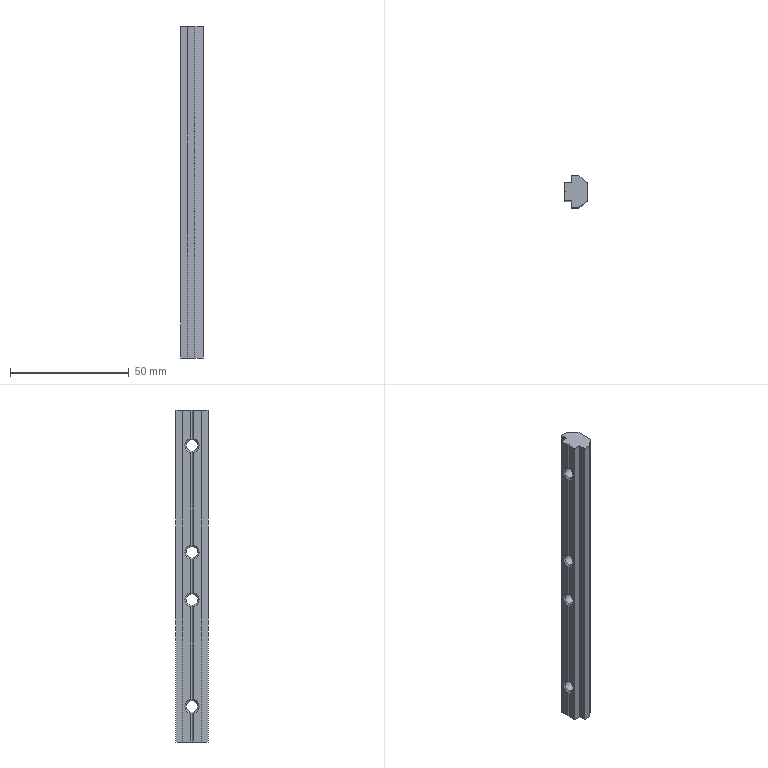Part | SolidWorks | features BaseBody 1 | 1 solid | 47 faces | box 9.5 x 13.5 x 140 mm | volume 13278 mm3 | plane 23 | cone 16 | cylinder 8 | commonest cylinder face diameters 4.917 x8
STEP:
#1=CARTESIAN_POINT('',(-0.5415,0.,-12.542));
#2=VERTEX_POINT('',#1);
#3=CARTESIAN_POINT('',(-0.5415,0.,-17.458));
#4=VERTEX_POINT('',#3);
#5=CARTESIAN_POINT('',(-0.5415,0.,-15.));
#6=DIRECTION('',(1.,0.,0.));
#7=DIRECTION('',(0.,0.,-1.));
#8=AXIS2_PLACEMENT_3D('',#5,#6,#7);
#9=CIRCLE('',#8,2.458);
#10=EDGE_CURVE('',#2,#4,#9,.T.);
#11=ORIENTED_EDGE('',*,*,#10,.F.);
#12=CARTESIAN_POINT('',(0.,0.,-12.));
#13=VERTEX_POINT('',#12);
#14=CARTESIAN_POINT('',(0.,0.,-12.));
#15=DIRECTION('',(0.7071,0.,0.7071));
#16=VECTOR('',#15,1000.);
#17=LINE('',#14,#16);
#18=EDGE_CURVE('',#2,#13,#17,.T.);
#19=ORIENTED_EDGE('',*,*,#18,.T.);
#20=CARTESIAN_POINT('',(0.,0.,-18.));
#21=VERTEX_POINT('',#20);
#22=CARTESIAN_POINT('',(0.,0.,-15.));
#23=DIRECTION('',(-1.,0.,0.));
#24=DIRECTION('',(0.,0.,-1.));
#25=AXIS2_PLACEMENT_3D('',#22,#23,#24);
#26=CIRCLE('',#25,3.);
#27=EDGE_CURVE('',#21,#13,#26,.T.);
#28=ORIENTED_EDGE('',*,*,#27,.F.);
#29=CARTESIAN_POINT('',(0.,0.,-18.));
#30=DIRECTION('',(0.7071,0.,-0.7071));
#31=VECTOR('',#30,1000.);
#32=LINE('',#29,#31);
#33=EDGE_CURVE('',#4,#21,#32,.T.);
#34=ORIENTED_EDGE('',*,*,#33,.F.);
#35=EDGE_LOOP('',(#11,#19,#28,#34));
#36=FACE_OUTER_BOUND('',#35,.T.);
#37=CARTESIAN_POINT('',(0.,0.,-15.));
#38=DIRECTION('',(1.,0.,0.));
#39=DIRECTION('',(0.,0.,-1.));
#40=AXIS2_PLACEMENT_3D('',#37,#38,#39);
#41=CONICAL_SURFACE('',#40,3.,0.7854);
#42=ADVANCED_FACE('',(#36),#41,.F.);
#43=CARTESIAN_POINT('',(-0.5415,0.,-57.541));
#44=VERTEX_POINT('',#43);
#45=CARTESIAN_POINT('',(-0.5415,0.,-62.459));
#46=VERTEX_POINT('',#45);
#47=CARTESIAN_POINT('',(-0.5415,0.,-60.));
#48=DIRECTION('',(1.,0.,0.));
#49=DIRECTION('',(0.,0.,-1.));
#50=AXIS2_PLACEMENT_3D('',#47,#48,#49);
#51=CIRCLE('',#50,2.459);
#52=EDGE_CURVE('',#44,#46,#51,.T.);
#53=ORIENTED_EDGE('',*,*,#52,.F.);
#54=CARTESIAN_POINT('',(0.,0.,-57.));
#55=VERTEX_POINT('',#54);
#56=CARTESIAN_POINT('',(0.,0.,-57.));
#57=DIRECTION('',(0.7071,0.,0.7071));
#58=VECTOR('',#57,1000.);
#59=LINE('',#56,#58);
#60=EDGE_CURVE('',#44,#55,#59,.T.);
#61=ORIENTED_EDGE('',*,*,#60,.T.);
#62=CARTESIAN_POINT('',(0.,0.,-63.));
#63=VERTEX_POINT('',#62);
#64=CARTESIAN_POINT('',(0.,0.,-60.));
#65=DIRECTION('',(-1.,0.,0.));
#66=DIRECTION('',(0.,0.,-1.));
#67=AXIS2_PLACEMENT_3D('',#64,#65,#66);
#68=CIRCLE('',#67,3.);
#69=EDGE_CURVE('',#63,#55,#68,.T.);
#70=ORIENTED_EDGE('',*,*,#69,.F.);
#71=CARTESIAN_POINT('',(0.,0.,-63.));
#72=DIRECTION('',(0.7071,0.,-0.7071));
#73=VECTOR('',#72,1000.);
#74=LINE('',#71,#73);
#75=EDGE_CURVE('',#46,#63,#74,.T.);
#76=ORIENTED_EDGE('',*,*,#75,.F.);
#77=EDGE_LOOP('',(#53,#61,#70,#76));
#78=FACE_OUTER_BOUND('',#77,.T.);
#79=CARTESIAN_POINT('',(0.,0.,-60.));
#80=DIRECTION('',(1.,0.,0.));
#81=DIRECTION('',(0.,0.,-1.));
#82=AXIS2_PLACEMENT_3D('',#79,#80,#81);
#83=CONICAL_SURFACE('',#82,3.,0.7854);
#84=ADVANCED_FACE('',(#78),#83,.F.);
#85=CARTESIAN_POINT('',(-0.5415,0.,-77.542));
#86=VERTEX_POINT('',#85);
#87=CARTESIAN_POINT('',(-0.5415,0.,-82.458));
#88=VERTEX_POINT('',#87);
#89=CARTESIAN_POINT('',(-0.5415,0.,-80.));
#90=DIRECTION('',(1.,0.,0.));
#91=DIRECTION('',(0.,0.,-1.));
#92=AXIS2_PLACEMENT_3D('',#89,#90,#91);
#93=CIRCLE('',#92,2.458);
#94=EDGE_CURVE('',#86,#88,#93,.T.);
#95=ORIENTED_EDGE('',*,*,#94,.F.);
#96=CARTESIAN_POINT('',(0.,0.,-77.));
#97=VERTEX_POINT('',#96);
#98=CARTESIAN_POINT('',(0.,0.,-77.));
#99=DIRECTION('',(0.7071,0.,0.7071));
#100=VECTOR('',#99,1000.);
#101=LINE('',#98,#100);
#102=EDGE_CURVE('',#86,#97,#101,.T.);
#103=ORIENTED_EDGE('',*,*,#102,.T.);
#104=CARTESIAN_POINT('',(0.,0.,-83.));
#105=VERTEX_POINT('',#104);
#106=CARTESIAN_POINT('',(0.,0.,-80.));
#107=DIRECTION('',(-1.,0.,0.));
#108=DIRECTION('',(0.,0.,-1.));
#109=AXIS2_PLACEMENT_3D('',#106,#107,#108);
#110=CIRCLE('',#109,3.);
#111=EDGE_CURVE('',#105,#97,#110,.T.);
#112=ORIENTED_EDGE('',*,*,#111,.F.);
#113=CARTESIAN_POINT('',(0.,0.,-83.));
#114=DIRECTION('',(0.7071,0.,-0.7071));
#115=VECTOR('',#114,1000.);
#116=LINE('',#113,#115);
#117=EDGE_CURVE('',#88,#105,#116,.T.);
#118=ORIENTED_EDGE('',*,*,#117,.F.);
#119=EDGE_LOOP('',(#95,#103,#112,#118));
#120=FACE_OUTER_BOUND('',#119,.T.);
#121=CARTESIAN_POINT('',(0.,0.,-80.));
#122=DIRECTION('',(1.,0.,0.));
#123=DIRECTION('',(0.,0.,-1.));
#124=AXIS2_PLACEMENT_3D('',#121,#122,#123);
#125=CONICAL_SURFACE('',#124,3.,0.7854);
#126=ADVANCED_FACE('',(#120),#125,.F.);
#127=CARTESIAN_POINT('',(-0.5415,0.,-122.541));
#128=VERTEX_POINT('',#127);
#129=CARTESIAN_POINT('',(-0.5415,0.,-127.459));
#130=VERTEX_POINT('',#129);
#131=CARTESIAN_POINT('',(-0.5415,0.,-125.));
#132=DIRECTION('',(1.,0.,0.));
#133=DIRECTION('',(0.,0.,-1.));
#134=AXIS2_PLACEMENT_3D('',#131,#132,#133);
#135=CIRCLE('',#134,2.459);
#136=EDGE_CURVE('',#128,#130,#135,.T.);
#137=ORIENTED_EDGE('',*,*,#136,.F.);
#138=CARTESIAN_POINT('',(0.,0.,-122.));
#139=VERTEX_POINT('',#138);
#140=CARTESIAN_POINT('',(0.,0.,-122.));
#141=DIRECTION('',(0.7071,0.,0.7071));
#142=VECTOR('',#141,1000.);
#143=LINE('',#140,#142);
#144=EDGE_CURVE('',#128,#139,#143,.T.);
#145=ORIENTED_EDGE('',*,*,#144,.T.);
#146=CARTESIAN_POINT('',(0.,0.,-128.));
#147=VERTEX_POINT('',#146);
#148=CARTESIAN_POINT('',(0.,0.,-125.));
#149=DIRECTION('',(-1.,0.,0.));
#150=DIRECTION('',(0.,0.,-1.));
#151=AXIS2_PLACEMENT_3D('',#148,#149,#150);
#152=CIRCLE('',#151,3.);
#153=EDGE_CURVE('',#147,#139,#152,.T.);
#154=ORIENTED_EDGE('',*,*,#153,.F.);
#155=CARTESIAN_POINT('',(0.,0.,-128.));
#156=DIRECTION('',(0.7071,0.,-0.7071));
#157=VECTOR('',#156,1000.);
#158=LINE('',#155,#157);
#159=EDGE_CURVE('',#130,#147,#158,.T.);
#160=ORIENTED_EDGE('',*,*,#159,.F.);
#161=EDGE_LOOP('',(#137,#145,#154,#160));
#162=FACE_OUTER_BOUND('',#161,.T.);
#163=CARTESIAN_POINT('',(0.,0.,-125.));
#164=DIRECTION('',(1.,0.,0.));
#165=DIRECTION('',(0.,0.,-1.));
#166=AXIS2_PLACEMENT_3D('',#163,#164,#165);
#167=CONICAL_SURFACE('',#166,3.,0.7854);
#168=ADVANCED_FACE('',(#162),#167,.F.);
#169=ORIENTED_EDGE('',*,*,#10,.T.);
#170=CARTESIAN_POINT('',(-8.959,0.,-17.458));
#171=VERTEX_POINT('',#170);
#172=CARTESIAN_POINT('',(0.,0.,-17.458));
#173=DIRECTION('',(-1.,0.,0.));
#174=VECTOR('',#173,1000.);
#175=LINE('',#172,#174);
#176=EDGE_CURVE('',#4,#171,#175,.T.);
#177=ORIENTED_EDGE('',*,*,#176,.T.);
#178=CARTESIAN_POINT('',(-8.959,0.,-12.542));
#179=VERTEX_POINT('',#178);
#180=CARTESIAN_POINT('',(-8.959,0.,-15.));
#181=DIRECTION('',(1.,0.,0.));
#182=DIRECTION('',(0.,0.,1.));
#183=AXIS2_PLACEMENT_3D('',#180,#181,#182);
#184=CIRCLE('',#183,2.458);
#185=EDGE_CURVE('',#179,#171,#184,.T.);
#186=ORIENTED_EDGE('',*,*,#185,.F.);
#187=CARTESIAN_POINT('',(0.,0.,-12.542));
#188=DIRECTION('',(-1.,0.,0.));
#189=VECTOR('',#188,1000.);
#190=LINE('',#187,#189);
#191=EDGE_CURVE('',#2,#179,#190,.T.);
#192=ORIENTED_EDGE('',*,*,#191,.F.);
#193=EDGE_LOOP('',(#169,#177,#186,#192));
#194=FACE_OUTER_BOUND('',#193,.T.);
#195=CARTESIAN_POINT('',(0.,0.,-15.));
#196=DIRECTION('',(-1.,0.,0.));
#197=DIRECTION('',(0.,0.,1.));
#198=AXIS2_PLACEMENT_3D('',#195,#196,#197);
#199=CYLINDRICAL_SURFACE('',#198,2.458);
#200=ADVANCED_FACE('',(#194),#199,.F.);
#201=ORIENTED_EDGE('',*,*,#52,.T.);
#202=CARTESIAN_POINT('',(-8.959,0.,-62.459));
#203=VERTEX_POINT('',#202);
#204=CARTESIAN_POINT('',(0.,0.,-62.459));
#205=DIRECTION('',(-1.,0.,0.));
#206=VECTOR('',#205,1000.);
#207=LINE('',#204,#206);
#208=EDGE_CURVE('',#46,#203,#207,.T.);
#209=ORIENTED_EDGE('',*,*,#208,.T.);
#210=CARTESIAN_POINT('',(-8.959,0.,-57.541));
#211=VERTEX_POINT('',#210);
#212=CARTESIAN_POINT('',(-8.959,0.,-60.));
#213=DIRECTION('',(1.,0.,0.));
#214=DIRECTION('',(0.,0.,1.));
#215=AXIS2_PLACEMENT_3D('',#212,#213,#214);
#216=CIRCLE('',#215,2.459);
#217=EDGE_CURVE('',#211,#203,#216,.T.);
#218=ORIENTED_EDGE('',*,*,#217,.F.);
#219=CARTESIAN_POINT('',(0.,0.,-57.541));
#220=DIRECTION('',(-1.,0.,0.));
#221=VECTOR('',#220,1000.);
#222=LINE('',#219,#221);
#223=EDGE_CURVE('',#44,#211,#222,.T.);
#224=ORIENTED_EDGE('',*,*,#223,.F.);
#225=EDGE_LOOP('',(#201,#209,#218,#224));
#226=FACE_OUTER_BOUND('',#225,.T.);
#227=CARTESIAN_POINT('',(0.,0.,-60.));
#228=DIRECTION('',(-1.,0.,0.));
#229=DIRECTION('',(0.,0.,1.));
#230=AXIS2_PLACEMENT_3D('',#227,#228,#229);
#231=CYLINDRICAL_SURFACE('',#230,2.459);
#232=ADVANCED_FACE('',(#226),#231,.F.);
#233=ORIENTED_EDGE('',*,*,#94,.T.);
#234=CARTESIAN_POINT('',(-8.959,0.,-82.459));
#235=VERTEX_POINT('',#234);
#236=CARTESIAN_POINT('',(0.,0.,-82.459));
#237=DIRECTION('',(-1.,0.,0.));
#238=VECTOR('',#237,1000.);
#239=LINE('',#236,#238);
#240=EDGE_CURVE('',#88,#235,#239,.T.);
#241=ORIENTED_EDGE('',*,*,#240,.T.);
#242=CARTESIAN_POINT('',(-8.959,0.,-77.541));
#243=VERTEX_POINT('',#242);
#244=CARTESIAN_POINT('',(-8.959,0.,-80.));
#245=DIRECTION('',(1.,0.,0.));
#246=DIRECTION('',(0.,0.,1.));
#247=AXIS2_PLACEMENT_3D('',#244,#245,#246);
#248=CIRCLE('',#247,2.459);
#249=EDGE_CURVE('',#243,#235,#248,.T.);
#250=ORIENTED_EDGE('',*,*,#249,.F.);
#251=CARTESIAN_POINT('',(0.,0.,-77.541));
#252=DIRECTION('',(-1.,0.,0.));
#253=VECTOR('',#252,1000.);
#254=LINE('',#251,#253);
#255=EDGE_CURVE('',#86,#243,#254,.T.);
#256=ORIENTED_EDGE('',*,*,#255,.F.);
#257=EDGE_LOOP('',(#233,#241,#250,#256));
#258=FACE_OUTER_BOUND('',#257,.T.);
#259=CARTESIAN_POINT('',(0.,0.,-80.));
#260=DIRECTION('',(-1.,0.,0.));
#261=DIRECTION('',(0.,0.,1.));
#262=AXIS2_PLACEMENT_3D('',#259,#260,#261);
#263=CYLINDRICAL_SURFACE('',#262,2.459);
#264=ADVANCED_FACE('',(#258),#263,.F.);
#265=ORIENTED_EDGE('',*,*,#136,.T.);
#266=CARTESIAN_POINT('',(-8.959,0.,-127.459));
#267=VERTEX_POINT('',#266);
#268=CARTESIAN_POINT('',(0.,0.,-127.459));
#269=DIRECTION('',(-1.,0.,0.));
#270=VECTOR('',#269,1000.);
#271=LINE('',#268,#270);
#272=EDGE_CURVE('',#130,#267,#271,.T.);
#273=ORIENTED_EDGE('',*,*,#272,.T.);
#274=CARTESIAN_POINT('',(-8.959,0.,-122.541));
#275=VERTEX_POINT('',#274);
#276=CARTESIAN_POINT('',(-8.959,0.,-125.));
#277=DIRECTION('',(1.,0.,0.));
#278=DIRECTION('',(0.,0.,1.));
#279=AXIS2_PLACEMENT_3D('',#276,#277,#278);
#280=CIRCLE('',#279,2.459);
#281=EDGE_CURVE('',#275,#267,#280,.T.);
#282=ORIENTED_EDGE('',*,*,#281,.F.);
#283=CARTESIAN_POINT('',(0.,0.,-122.541));
#284=DIRECTION('',(-1.,0.,0.));
#285=VECTOR('',#284,1000.);
#286=LINE('',#283,#285);
#287=EDGE_CURVE('',#128,#275,#286,.T.);
#288=ORIENTED_EDGE('',*,*,#287,.F.);
#289=EDGE_LOOP('',(#265,#273,#282,#288));
#290=FACE_OUTER_BOUND('',#289,.T.);
#291=CARTESIAN_POINT('',(0.,0.,-125.));
#292=DIRECTION('',(-1.,0.,0.));
#293=DIRECTION('',(0.,0.,1.));
#294=AXIS2_PLACEMENT_3D('',#291,#292,#293);
#295=CYLINDRICAL_SURFACE('',#294,2.459);
#296=ADVANCED_FACE('',(#290),#295,.F.);
#297=ORIENTED_EDGE('',*,*,#249,.T.);
#298=CARTESIAN_POINT('',(-9.,0.,-82.5));
#299=VERTEX_POINT('',#298);
#300=CARTESIAN_POINT('',(-9.5,0.,-83.));
#301=DIRECTION('',(-0.7071,0.,-0.7071));
#302=VECTOR('',#301,1000.);
#303=LINE('',#300,#302);
#304=EDGE_CURVE('',#235,#299,#303,.T.);
#305=ORIENTED_EDGE('',*,*,#304,.T.);
#306=CARTESIAN_POINT('',(-9.5,-0.5,-82.958));
#307=VERTEX_POINT('',#306);
#308=CARTESIAN_POINT('',(-9.5,-0.5,-82.958));
#309=CARTESIAN_POINT('',(-9.319,-0.3193,-82.805));
#310=CARTESIAN_POINT('',(-9.153,-0.1527,-82.653));
#311=CARTESIAN_POINT('',(-9.,0.,-82.5));
#312=B_SPLINE_CURVE_WITH_KNOTS('',3,(#308,#309,#310,#311),.UNSPECIFIED.,.F.,.F.,(4,4),(0.,1.),.UNSPECIFIED.);
#313=EDGE_CURVE('',#307,#299,#312,.T.);
#314=ORIENTED_EDGE('',*,*,#313,.F.);
#315=CARTESIAN_POINT('',(-9.5,-0.5,-77.042));
#316=VERTEX_POINT('',#315);
#317=CARTESIAN_POINT('',(-9.5,0.,-80.));
#318=DIRECTION('',(1.,0.,0.));
#319=DIRECTION('',(0.,0.,1.));
#320=AXIS2_PLACEMENT_3D('',#317,#318,#319);
#321=CIRCLE('',#320,3.);
#322=EDGE_CURVE('',#316,#307,#321,.T.);
#323=ORIENTED_EDGE('',*,*,#322,.F.);
#324=CARTESIAN_POINT('',(-9.,0.,-77.5));
#325=VERTEX_POINT('',#324);
#326=CARTESIAN_POINT('',(-9.,0.,-77.5));
#327=CARTESIAN_POINT('',(-9.153,-0.1527,-77.347));
#328=CARTESIAN_POINT('',(-9.319,-0.3193,-77.195));
#329=CARTESIAN_POINT('',(-9.5,-0.5,-77.042));
#330=B_SPLINE_CURVE_WITH_KNOTS('',3,(#326,#327,#328,#329),.UNSPECIFIED.,.F.,.F.,(4,4),(0.,1.),.UNSPECIFIED.);
#331=EDGE_CURVE('',#325,#316,#330,.T.);
#332=ORIENTED_EDGE('',*,*,#331,.F.);
#333=CARTESIAN_POINT('',(-9.5,0.,-77.));
#334=DIRECTION('',(-0.7071,0.,0.7071));
#335=VECTOR('',#334,1000.);
#336=LINE('',#333,#335);
#337=EDGE_CURVE('',#243,#325,#336,.T.);
#338=ORIENTED_EDGE('',*,*,#337,.F.);
#339=EDGE_LOOP('',(#297,#305,#314,#323,#332,#338));
#340=FACE_OUTER_BOUND('',#339,.T.);
#341=CARTESIAN_POINT('',(-9.5,0.,-80.));
#342=DIRECTION('',(-1.,0.,0.));
#343=DIRECTION('',(0.,0.,1.));
#344=AXIS2_PLACEMENT_3D('',#341,#342,#343);
#345=CONICAL_SURFACE('',#344,3.,0.7854);
#346=ADVANCED_FACE('',(#340),#345,.F.);
#347=ORIENTED_EDGE('',*,*,#217,.T.);
#348=CARTESIAN_POINT('',(-9.,0.,-62.5));
#349=VERTEX_POINT('',#348);
#350=CARTESIAN_POINT('',(-9.5,0.,-63.));
#351=DIRECTION('',(-0.7071,0.,-0.7071));
#352=VECTOR('',#351,1000.);
#353=LINE('',#350,#352);
#354=EDGE_CURVE('',#203,#349,#353,.T.);
#355=ORIENTED_EDGE('',*,*,#354,.T.);
#356=CARTESIAN_POINT('',(-9.5,-0.5,-62.958));
#357=VERTEX_POINT('',#356);
#358=CARTESIAN_POINT('',(-9.5,-0.5,-62.958));
#359=CARTESIAN_POINT('',(-9.319,-0.3193,-62.805));
#360=CARTESIAN_POINT('',(-9.153,-0.1527,-62.653));
#361=CARTESIAN_POINT('',(-9.,0.,-62.5));
#362=B_SPLINE_CURVE_WITH_KNOTS('',3,(#358,#359,#360,#361),.UNSPECIFIED.,.F.,.F.,(4,4),(0.,1.),.UNSPECIFIED.);
#363=EDGE_CURVE('',#357,#349,#362,.T.);
#364=ORIENTED_EDGE('',*,*,#363,.F.);
#365=CARTESIAN_POINT('',(-9.5,-0.5,-57.042));
#366=VERTEX_POINT('',#365);
#367=CARTESIAN_POINT('',(-9.5,0.,-60.));
#368=DIRECTION('',(1.,0.,0.));
#369=DIRECTION('',(0.,0.,1.));
#370=AXIS2_PLACEMENT_3D('',#367,#368,#369);
#371=CIRCLE('',#370,3.);
#372=EDGE_CURVE('',#366,#357,#371,.T.);
#373=ORIENTED_EDGE('',*,*,#372,.F.);
#374=CARTESIAN_POINT('',(-9.,0.,-57.5));
#375=VERTEX_POINT('',#374);
#376=CARTESIAN_POINT('',(-9.,0.,-57.5));
#377=CARTESIAN_POINT('',(-9.153,-0.1527,-57.347));
#378=CARTESIAN_POINT('',(-9.319,-0.3193,-57.195));
#379=CARTESIAN_POINT('',(-9.5,-0.5,-57.042));
#380=B_SPLINE_CURVE_WITH_KNOTS('',3,(#376,#377,#378,#379),.UNSPECIFIED.,.F.,.F.,(4,4),(0.,1.),.UNSPECIFIED.);
#381=EDGE_CURVE('',#375,#366,#380,.T.);
#382=ORIENTED_EDGE('',*,*,#381,.F.);
#383=CARTESIAN_POINT('',(-9.5,0.,-57.));
#384=DIRECTION('',(-0.7071,0.,0.7071));
#385=VECTOR('',#384,1000.);
#386=LINE('',#383,#385);
#387=EDGE_CURVE('',#211,#375,#386,.T.);
#388=ORIENTED_EDGE('',*,*,#387,.F.);
#389=EDGE_LOOP('',(#347,#355,#364,#373,#382,#388));
#390=FACE_OUTER_BOUND('',#389,.T.);
#391=CARTESIAN_POINT('',(-9.5,0.,-60.));
#392=DIRECTION('',(-1.,0.,0.));
#393=DIRECTION('',(0.,0.,1.));
#394=AXIS2_PLACEMENT_3D('',#391,#392,#393);
#395=CONICAL_SURFACE('',#394,3.,0.7854);
#396=ADVANCED_FACE('',(#390),#395,.F.);
#397=ORIENTED_EDGE('',*,*,#185,.T.);
#398=CARTESIAN_POINT('',(-9.,0.,-17.5));
#399=VERTEX_POINT('',#398);
#400=CARTESIAN_POINT('',(-9.5,0.,-18.));
#401=DIRECTION('',(-0.7071,0.,-0.7071));
#402=VECTOR('',#401,1000.);
#403=LINE('',#400,#402);
#404=EDGE_CURVE('',#171,#399,#403,.T.);
#405=ORIENTED_EDGE('',*,*,#404,.T.);
#406=CARTESIAN_POINT('',(-9.5,-0.5,-17.958));
#407=VERTEX_POINT('',#406);
#408=CARTESIAN_POINT('',(-9.5,-0.5,-17.958));
#409=CARTESIAN_POINT('',(-9.319,-0.3193,-17.805));
#410=CARTESIAN_POINT('',(-9.153,-0.1527,-17.653));
#411=CARTESIAN_POINT('',(-9.,0.,-17.5));
#412=B_SPLINE_CURVE_WITH_KNOTS('',3,(#408,#409,#410,#411),.UNSPECIFIED.,.F.,.F.,(4,4),(0.,1.),.UNSPECIFIED.);
#413=EDGE_CURVE('',#407,#399,#412,.T.);
#414=ORIENTED_EDGE('',*,*,#413,.F.);
#415=CARTESIAN_POINT('',(-9.5,-0.5,-12.042));
#416=VERTEX_POINT('',#415);
#417=CARTESIAN_POINT('',(-9.5,0.,-15.));
#418=DIRECTION('',(1.,0.,0.));
#419=DIRECTION('',(0.,0.,1.));
#420=AXIS2_PLACEMENT_3D('',#417,#418,#419);
#421=CIRCLE('',#420,3.);
#422=EDGE_CURVE('',#416,#407,#421,.T.);
#423=ORIENTED_EDGE('',*,*,#422,.F.);
#424=CARTESIAN_POINT('',(-9.,0.,-12.5));
#425=VERTEX_POINT('',#424);
#426=CARTESIAN_POINT('',(-9.,0.,-12.5));
#427=CARTESIAN_POINT('',(-9.153,-0.1527,-12.347));
#428=CARTESIAN_POINT('',(-9.319,-0.3193,-12.195));
#429=CARTESIAN_POINT('',(-9.5,-0.5,-12.042));
#430=B_SPLINE_CURVE_WITH_KNOTS('',3,(#426,#427,#428,#429),.UNSPECIFIED.,.F.,.F.,(4,4),(0.,1.),.UNSPECIFIED.);
#431=EDGE_CURVE('',#425,#416,#430,.T.);
#432=ORIENTED_EDGE('',*,*,#431,.F.);
#433=CARTESIAN_POINT('',(-9.5,0.,-12.));
#434=DIRECTION('',(-0.7071,0.,0.7071));
#435=VECTOR('',#434,1000.);
#436=LINE('',#433,#435);
#437=EDGE_CURVE('',#179,#425,#436,.T.);
#438=ORIENTED_EDGE('',*,*,#437,.F.);
#439=EDGE_LOOP('',(#397,#405,#414,#423,#432,#438));
#440=FACE_OUTER_BOUND('',#439,.T.);
#441=CARTESIAN_POINT('',(-9.5,0.,-15.));
#442=DIRECTION('',(-1.,0.,0.));
#443=DIRECTION('',(0.,0.,1.));
#444=AXIS2_PLACEMENT_3D('',#441,#442,#443);
#445=CONICAL_SURFACE('',#444,3.,0.7854);
#446=ADVANCED_FACE('',(#440),#445,.F.);
#447=ORIENTED_EDGE('',*,*,#281,.T.);
#448=CARTESIAN_POINT('',(-9.,0.,-127.5));
#449=VERTEX_POINT('',#448);
#450=CARTESIAN_POINT('',(-9.5,0.,-128.));
#451=DIRECTION('',(-0.7071,0.,-0.7071));
#452=VECTOR('',#451,1000.);
#453=LINE('',#450,#452);
#454=EDGE_CURVE('',#267,#449,#453,.T.);
#455=ORIENTED_EDGE('',*,*,#454,.T.);
#456=CARTESIAN_POINT('',(-9.5,-0.5,-127.958));
#457=VERTEX_POINT('',#456);
#458=CARTESIAN_POINT('',(-9.5,-0.5,-127.958));
#459=CARTESIAN_POINT('',(-9.319,-0.3193,-127.805));
#460=CARTESIAN_POINT('',(-9.153,-0.1527,-127.653));
#461=CARTESIAN_POINT('',(-9.,0.,-127.5));
#462=B_SPLINE_CURVE_WITH_KNOTS('',3,(#458,#459,#460,#461),.UNSPECIFIED.,.F.,.F.,(4,4),(0.,1.),.UNSPECIFIED.);
#463=EDGE_CURVE('',#457,#449,#462,.T.);
#464=ORIENTED_EDGE('',*,*,#463,.F.);
#465=CARTESIAN_POINT('',(-9.5,-0.5,-122.042));
#466=VERTEX_POINT('',#465);
#467=CARTESIAN_POINT('',(-9.5,0.,-125.));
#468=DIRECTION('',(1.,0.,0.));
#469=DIRECTION('',(0.,0.,1.));
#470=AXIS2_PLACEMENT_3D('',#467,#468,#469);
#471=CIRCLE('',#470,3.);
#472=EDGE_CURVE('',#466,#457,#471,.T.);
#473=ORIENTED_EDGE('',*,*,#472,.F.);
#474=CARTESIAN_POINT('',(-9.,0.,-122.5));
#475=VERTEX_POINT('',#474);
#476=CARTESIAN_POINT('',(-9.,0.,-122.5));
#477=CARTESIAN_POINT('',(-9.153,-0.1527,-122.347));
#478=CARTESIAN_POINT('',(-9.319,-0.3193,-122.195));
#479=CARTESIAN_POINT('',(-9.5,-0.5,-122.042));
#480=B_SPLINE_CURVE_WITH_KNOTS('',3,(#476,#477,#478,#479),.UNSPECIFIED.,.F.,.F.,(4,4),(0.,1.),.UNSPECIFIED.);
#481=EDGE_CURVE('',#475,#466,#480,.T.);
#482=ORIENTED_EDGE('',*,*,#481,.F.);
#483=CARTESIAN_POINT('',(-9.5,0.,-122.));
#484=DIRECTION('',(-0.7071,0.,0.7071));
#485=VECTOR('',#484,1000.);
#486=LINE('',#483,#485);
#487=EDGE_CURVE('',#275,#475,#486,.T.);
#488=ORIENTED_EDGE('',*,*,#487,.F.);
#489=EDGE_LOOP('',(#447,#455,#464,#473,#482,#488));
#490=FACE_OUTER_BOUND('',#489,.T.);
#491=CARTESIAN_POINT('',(-9.5,0.,-125.));
#492=DIRECTION('',(-1.,0.,0.));
#493=DIRECTION('',(0.,0.,1.));
#494=AXIS2_PLACEMENT_3D('',#491,#492,#493);
#495=CONICAL_SURFACE('',#494,3.,0.7854);
#496=ADVANCED_FACE('',(#490),#495,.F.);
#497=CARTESIAN_POINT('',(0.,-3.675,-140.));
#498=VERTEX_POINT('',#497);
#499=CARTESIAN_POINT('',(0.,3.675,-140.));
#500=VERTEX_POINT('',#499);
#501=CARTESIAN_POINT('',(0.,-3.675,-140.));
#502=DIRECTION('',(0.,1.,0.));
#503=VECTOR('',#502,1000.);
#504=LINE('',#501,#503);
#505=EDGE_CURVE('',#498,#500,#504,.T.);
#506=ORIENTED_EDGE('',*,*,#505,.T.);
#507=CARTESIAN_POINT('',(0.,3.675,0.));
#508=VERTEX_POINT('',#507);
#509=CARTESIAN_POINT('',(0.,3.675,-140.));
#510=DIRECTION('',(0.,0.,1.));
#511=VECTOR('',#510,1000.);
#512=LINE('',#509,#511);
#513=EDGE_CURVE('',#500,#508,#512,.T.);
#514=ORIENTED_EDGE('',*,*,#513,.T.);
#515=CARTESIAN_POINT('',(0.,-3.675,0.));
#516=VERTEX_POINT('',#515);
#517=CARTESIAN_POINT('',(0.,-3.675,0.));
#518=DIRECTION('',(0.,-1.,0.));
#519=VECTOR('',#518,1000.);
#520=LINE('',#517,#519);
#521=EDGE_CURVE('',#508,#516,#520,.T.);
#522=ORIENTED_EDGE('',*,*,#521,.T.);
#523=CARTESIAN_POINT('',(0.,-3.675,-140.));
#524=DIRECTION('',(0.,0.,-1.));
#525=VECTOR('',#524,1000.);
#526=LINE('',#523,#525);
#527=EDGE_CURVE('',#516,#498,#526,.T.);
#528=ORIENTED_EDGE('',*,*,#527,.T.);
#529=EDGE_LOOP('',(#506,#514,#522,#528));
#530=FACE_OUTER_BOUND('',#529,.T.);
#531=ORIENTED_EDGE('',*,*,#27,.T.);
#532=CARTESIAN_POINT('',(0.,0.,-15.));
#533=DIRECTION('',(-1.,0.,0.));
#534=DIRECTION('',(0.,0.,-1.));
#535=AXIS2_PLACEMENT_3D('',#532,#533,#534);
#536=CIRCLE('',#535,3.);
#537=EDGE_CURVE('',#13,#21,#536,.T.);
#538=ORIENTED_EDGE('',*,*,#537,.T.);
#539=EDGE_LOOP('',(#531,#538));
#540=FACE_BOUND('',#539,.T.);
#541=ORIENTED_EDGE('',*,*,#69,.T.);
#542=CARTESIAN_POINT('',(0.,0.,-60.));
#543=DIRECTION('',(-1.,0.,0.));
#544=DIRECTION('',(0.,0.,-1.));
#545=AXIS2_PLACEMENT_3D('',#542,#543,#544);
#546=CIRCLE('',#545,3.);
#547=EDGE_CURVE('',#55,#63,#546,.T.);
#548=ORIENTED_EDGE('',*,*,#547,.T.);
#549=EDGE_LOOP('',(#541,#548));
#550=FACE_BOUND('',#549,.T.);
#551=ORIENTED_EDGE('',*,*,#111,.T.);
#552=CARTESIAN_POINT('',(0.,0.,-80.));
#553=DIRECTION('',(-1.,0.,0.));
#554=DIRECTION('',(0.,0.,-1.));
#555=AXIS2_PLACEMENT_3D('',#552,#553,#554);
#556=CIRCLE('',#555,3.);
#557=EDGE_CURVE('',#97,#105,#556,.T.);
#558=ORIENTED_EDGE('',*,*,#557,.T.);
#559=EDGE_LOOP('',(#551,#558));
#560=FACE_BOUND('',#559,.T.);
#561=ORIENTED_EDGE('',*,*,#153,.T.);
#562=CARTESIAN_POINT('',(0.,0.,-125.));
#563=DIRECTION('',(-1.,0.,0.));
#564=DIRECTION('',(0.,0.,-1.));
#565=AXIS2_PLACEMENT_3D('',#562,#563,#564);
#566=CIRCLE('',#565,3.);
#567=EDGE_CURVE('',#139,#147,#566,.T.);
#568=ORIENTED_EDGE('',*,*,#567,.T.);
#569=EDGE_LOOP('',(#561,#568));
#570=FACE_BOUND('',#569,.T.);
#571=CARTESIAN_POINT('',(0.,-3.675,-140.));
#572=DIRECTION('',(1.,0.,0.));
#573=DIRECTION('',(0.,0.,-1.));
#574=AXIS2_PLACEMENT_3D('',#571,#572,#573);
#575=PLANE('',#574);
#576=ADVANCED_FACE('',(#530,#540,#550,#560,#570),#575,.T.);
#577=CARTESIAN_POINT('',(-3.514,6.75,-140.));
#578=VERTEX_POINT('',#577);
#579=CARTESIAN_POINT('',(0.,3.675,-140.));
#580=DIRECTION('',(-0.7526,0.6585,0.));
#581=VECTOR('',#580,1000.);
#582=LINE('',#579,#581);
#583=EDGE_CURVE('',#500,#578,#582,.T.);
#584=ORIENTED_EDGE('',*,*,#583,.T.);
#585=CARTESIAN_POINT('',(-3.514,6.75,0.));
#586=VERTEX_POINT('',#585);
#587=CARTESIAN_POINT('',(-3.514,6.75,-140.));
#588=DIRECTION('',(0.,0.,1.));
#589=VECTOR('',#588,1000.);
#590=LINE('',#587,#589);
#591=EDGE_CURVE('',#578,#586,#590,.T.);
#592=ORIENTED_EDGE('',*,*,#591,.T.);
#593=CARTESIAN_POINT('',(0.,3.675,0.));
#594=DIRECTION('',(0.7526,-0.6585,0.));
#595=VECTOR('',#594,1000.);
#596=LINE('',#593,#595);
#597=EDGE_CURVE('',#586,#508,#596,.T.);
#598=ORIENTED_EDGE('',*,*,#597,.T.);
#599=ORIENTED_EDGE('',*,*,#513,.F.);
#600=EDGE_LOOP('',(#584,#592,#598,#599));
#601=FACE_OUTER_BOUND('',#600,.T.);
#602=CARTESIAN_POINT('',(0.,3.675,-140.));
#603=DIRECTION('',(0.6585,0.7526,0.));
#604=DIRECTION('',(-0.7526,0.6585,0.));
#605=AXIS2_PLACEMENT_3D('',#602,#603,#604);
#606=PLANE('',#605);
#607=ADVANCED_FACE('',(#601),#606,.T.);
#608=CARTESIAN_POINT('',(-6.5,6.75,-140.));
#609=VERTEX_POINT('',#608);
#610=CARTESIAN_POINT('',(-6.5,3.9,-140.));
#611=VERTEX_POINT('',#610);
#612=CARTESIAN_POINT('',(-6.5,0.,-140.));
#613=DIRECTION('',(0.,-1.,0.));
#614=VECTOR('',#613,1000.);
#615=LINE('',#612,#614);
#616=EDGE_CURVE('',#609,#611,#615,.T.);
#617=ORIENTED_EDGE('',*,*,#616,.F.);
#618=CARTESIAN_POINT('',(0.,6.75,-140.));
#619=DIRECTION('',(-1.,0.,0.));
#620=VECTOR('',#619,1000.);
#621=LINE('',#618,#620);
#622=EDGE_CURVE('',#578,#609,#621,.T.);
#623=ORIENTED_EDGE('',*,*,#622,.F.);
#624=ORIENTED_EDGE('',*,*,#583,.F.);
#625=ORIENTED_EDGE('',*,*,#505,.F.);
#626=CARTESIAN_POINT('',(-3.514,-6.75,-140.));
#627=VERTEX_POINT('',#626);
#628=CARTESIAN_POINT('',(-3.514,-6.75,-140.));
#629=DIRECTION('',(0.7526,0.6585,0.));
#630=VECTOR('',#629,1000.);
#631=LINE('',#628,#630);
#632=EDGE_CURVE('',#627,#498,#631,.T.);
#633=ORIENTED_EDGE('',*,*,#632,.F.);
#634=CARTESIAN_POINT('',(-6.5,-6.75,-140.));
#635=VERTEX_POINT('',#634);
#636=CARTESIAN_POINT('',(0.,-6.75,-140.));
#637=DIRECTION('',(1.,0.,0.));
#638=VECTOR('',#637,1000.);
#639=LINE('',#636,#638);
#640=EDGE_CURVE('',#635,#627,#639,.T.);
#641=ORIENTED_EDGE('',*,*,#640,.F.);
#642=CARTESIAN_POINT('',(-6.5,-3.9,-140.));
#643=VERTEX_POINT('',#642);
#644=CARTESIAN_POINT('',(-6.5,0.,-140.));
#645=DIRECTION('',(0.,-1.,0.));
#646=VECTOR('',#645,1000.);
#647=LINE('',#644,#646);
#648=EDGE_CURVE('',#643,#635,#647,.T.);
#649=ORIENTED_EDGE('',*,*,#648,.F.);
#650=CARTESIAN_POINT('',(-9.5,-3.9,-140.));
#651=VERTEX_POINT('',#650);
#652=CARTESIAN_POINT('',(0.,-3.9,-140.));
#653=DIRECTION('',(1.,0.,0.));
#654=VECTOR('',#653,1000.);
#655=LINE('',#652,#654);
#656=EDGE_CURVE('',#651,#643,#655,.T.);
#657=ORIENTED_EDGE('',*,*,#656,.F.);
#658=CARTESIAN_POINT('',(-9.5,-0.5,-140.));
#659=VERTEX_POINT('',#658);
#660=CARTESIAN_POINT('',(-9.5,0.,-140.));
#661=DIRECTION('',(0.,-1.,0.));
#662=VECTOR('',#661,1000.);
#663=LINE('',#660,#662);
#664=EDGE_CURVE('',#659,#651,#663,.T.);
#665=ORIENTED_EDGE('',*,*,#664,.F.);
#666=CARTESIAN_POINT('',(-9.,0.,-140.));
#667=VERTEX_POINT('',#666);
#668=CARTESIAN_POINT('',(-9.,0.,-140.));
#669=DIRECTION('',(-0.7071,-0.7071,0.));
#670=VECTOR('',#669,1000.);
#671=LINE('',#668,#670);
#672=EDGE_CURVE('',#667,#659,#671,.T.);
#673=ORIENTED_EDGE('',*,*,#672,.F.);
#674=CARTESIAN_POINT('',(-9.5,0.5,-140.));
#675=VERTEX_POINT('',#674);
#676=CARTESIAN_POINT('',(-9.5,0.5,-140.));
#677=DIRECTION('',(0.7071,-0.7071,0.));
#678=VECTOR('',#677,1000.);
#679=LINE('',#676,#678);
#680=EDGE_CURVE('',#675,#667,#679,.T.);
#681=ORIENTED_EDGE('',*,*,#680,.F.);
#682=CARTESIAN_POINT('',(-9.5,3.9,-140.));
#683=VERTEX_POINT('',#682);
#684=CARTESIAN_POINT('',(-9.5,0.,-140.));
#685=DIRECTION('',(0.,-1.,0.));
#686=VECTOR('',#685,1000.);
#687=LINE('',#684,#686);
#688=EDGE_CURVE('',#683,#675,#687,.T.);
#689=ORIENTED_EDGE('',*,*,#688,.F.);
#690=CARTESIAN_POINT('',(0.,3.9,-140.));
#691=DIRECTION('',(-1.,0.,0.));
#692=VECTOR('',#691,1000.);
#693=LINE('',#690,#692);
#694=EDGE_CURVE('',#611,#683,#693,.T.);
#695=ORIENTED_EDGE('',*,*,#694,.F.);
#696=EDGE_LOOP('',(#617,#623,#624,#625,#633,#641,#649,#657,#665,#673,#681,#689,#695));
#697=FACE_OUTER_BOUND('',#696,.T.);
#698=CARTESIAN_POINT('',(0.,0.,-140.));
#699=DIRECTION('',(0.,0.,1.));
#700=DIRECTION('',(1.,0.,0.));
#701=AXIS2_PLACEMENT_3D('',#698,#699,#700);
#702=PLANE('',#701);
#703=ADVANCED_FACE('',(#697),#702,.F.);
#704=ORIENTED_EDGE('',*,*,#632,.T.);
#705=ORIENTED_EDGE('',*,*,#527,.F.);
#706=CARTESIAN_POINT('',(-3.514,-6.75,0.));
#707=VERTEX_POINT('',#706);
#708=CARTESIAN_POINT('',(-3.514,-6.75,0.));
#709=DIRECTION('',(-0.7526,-0.6585,0.));
#710=VECTOR('',#709,1000.);
#711=LINE('',#708,#710);
#712=EDGE_CURVE('',#516,#707,#711,.T.);
#713=ORIENTED_EDGE('',*,*,#712,.T.);
#714=CARTESIAN_POINT('',(-3.514,-6.75,-140.));
#715=DIRECTION('',(0.,0.,-1.));
#716=VECTOR('',#715,1000.);
#717=LINE('',#714,#716);
#718=EDGE_CURVE('',#707,#627,#717,.T.);
#719=ORIENTED_EDGE('',*,*,#718,.T.);
#720=EDGE_LOOP('',(#704,#705,#713,#719));
#721=FACE_OUTER_BOUND('',#720,.T.);
#722=CARTESIAN_POINT('',(-3.514,-6.75,-140.));
#723=DIRECTION('',(0.6585,-0.7526,0.));
#724=DIRECTION('',(0.7526,0.6585,0.));
#725=AXIS2_PLACEMENT_3D('',#722,#723,#724);
#726=PLANE('',#725);
#727=ADVANCED_FACE('',(#721),#726,.T.);
#728=CARTESIAN_POINT('',(-6.5,6.75,0.));
#729=VERTEX_POINT('',#728);
#730=CARTESIAN_POINT('',(0.,6.75,0.));
#731=DIRECTION('',(-1.,0.,0.));
#732=VECTOR('',#731,1000.);
#733=LINE('',#730,#732);
#734=EDGE_CURVE('',#586,#729,#733,.T.);
#735=ORIENTED_EDGE('',*,*,#734,.T.);
#736=CARTESIAN_POINT('',(-6.5,3.9,0.));
#737=VERTEX_POINT('',#736);
#738=CARTESIAN_POINT('',(-6.5,0.,0.));
#739=DIRECTION('',(0.,-1.,0.));
#740=VECTOR('',#739,1000.);
#741=LINE('',#738,#740);
#742=EDGE_CURVE('',#729,#737,#741,.T.);
#743=ORIENTED_EDGE('',*,*,#742,.T.);
#744=CARTESIAN_POINT('',(-9.5,3.9,0.));
#745=VERTEX_POINT('',#744);
#746=CARTESIAN_POINT('',(0.,3.9,0.));
#747=DIRECTION('',(-1.,0.,0.));
#748=VECTOR('',#747,1000.);
#749=LINE('',#746,#748);
#750=EDGE_CURVE('',#737,#745,#749,.T.);
#751=ORIENTED_EDGE('',*,*,#750,.T.);
#752=CARTESIAN_POINT('',(-9.5,0.5,0.));
#753=VERTEX_POINT('',#752);
#754=CARTESIAN_POINT('',(-9.5,0.,0.));
#755=DIRECTION('',(0.,-1.,0.));
#756=VECTOR('',#755,1000.);
#757=LINE('',#754,#756);
#758=EDGE_CURVE('',#745,#753,#757,.T.);
#759=ORIENTED_EDGE('',*,*,#758,.T.);
#760=CARTESIAN_POINT('',(-9.,0.,0.));
#761=VERTEX_POINT('',#760);
#762=CARTESIAN_POINT('',(-9.5,0.5,0.));
#763=DIRECTION('',(-0.7071,0.7071,0.));
#764=VECTOR('',#763,1000.);
#765=LINE('',#762,#764);
#766=EDGE_CURVE('',#761,#753,#765,.T.);
#767=ORIENTED_EDGE('',*,*,#766,.F.);
#768=CARTESIAN_POINT('',(-9.5,-0.5,0.));
#769=VERTEX_POINT('',#768);
#770=CARTESIAN_POINT('',(-9.,0.,0.));
#771=DIRECTION('',(0.7071,0.7071,0.));
#772=VECTOR('',#771,1000.);
#773=LINE('',#770,#772);
#774=EDGE_CURVE('',#769,#761,#773,.T.);
#775=ORIENTED_EDGE('',*,*,#774,.F.);
#776=CARTESIAN_POINT('',(-9.5,-3.9,0.));
#777=VERTEX_POINT('',#776);
#778=CARTESIAN_POINT('',(-9.5,0.,0.));
#779=DIRECTION('',(0.,-1.,0.));
#780=VECTOR('',#779,1000.);
#781=LINE('',#778,#780);
#782=EDGE_CURVE('',#769,#777,#781,.T.);
#783=ORIENTED_EDGE('',*,*,#782,.T.);
#784=CARTESIAN_POINT('',(-6.5,-3.9,0.));
#785=VERTEX_POINT('',#784);
#786=CARTESIAN_POINT('',(0.,-3.9,0.));
#787=DIRECTION('',(1.,0.,0.));
#788=VECTOR('',#787,1000.);
#789=LINE('',#786,#788);
#790=EDGE_CURVE('',#777,#785,#789,.T.);
#791=ORIENTED_EDGE('',*,*,#790,.T.);
#792=CARTESIAN_POINT('',(-6.5,-6.75,0.));
#793=VERTEX_POINT('',#792);
#794=CARTESIAN_POINT('',(-6.5,0.,0.));
#795=DIRECTION('',(0.,-1.,0.));
#796=VECTOR('',#795,1000.);
#797=LINE('',#794,#796);
#798=EDGE_CURVE('',#785,#793,#797,.T.);
#799=ORIENTED_EDGE('',*,*,#798,.T.);
#800=CARTESIAN_POINT('',(0.,-6.75,0.));
#801=DIRECTION('',(1.,0.,0.));
#802=VECTOR('',#801,1000.);
#803=LINE('',#800,#802);
#804=EDGE_CURVE('',#793,#707,#803,.T.);
#805=ORIENTED_EDGE('',*,*,#804,.T.);
#806=ORIENTED_EDGE('',*,*,#712,.F.);
#807=ORIENTED_EDGE('',*,*,#521,.F.);
#808=ORIENTED_EDGE('',*,*,#597,.F.);
#809=EDGE_LOOP('',(#735,#743,#751,#759,#767,#775,#783,#791,#799,#805,#806,#807,#808));
#810=FACE_OUTER_BOUND('',#809,.T.);
#811=CARTESIAN_POINT('',(0.,0.,0.));
#812=DIRECTION('',(0.,0.,1.));
#813=DIRECTION('',(1.,0.,0.));
#814=AXIS2_PLACEMENT_3D('',#811,#812,#813);
#815=PLANE('',#814);
#816=ADVANCED_FACE('',(#810),#815,.T.);
#817=ORIENTED_EDGE('',*,*,#18,.F.);
#818=CARTESIAN_POINT('',(-0.5415,0.,-15.));
#819=DIRECTION('',(1.,0.,0.));
#820=DIRECTION('',(0.,0.,-1.));
#821=AXIS2_PLACEMENT_3D('',#818,#819,#820);
#822=CIRCLE('',#821,2.458);
#823=EDGE_CURVE('',#4,#2,#822,.T.);
#824=ORIENTED_EDGE('',*,*,#823,.F.);
#825=ORIENTED_EDGE('',*,*,#33,.T.);
#826=ORIENTED_EDGE('',*,*,#537,.F.);
#827=EDGE_LOOP('',(#817,#824,#825,#826));
#828=FACE_OUTER_BOUND('',#827,.T.);
#829=CARTESIAN_POINT('',(0.,0.,-15.));
#830=DIRECTION('',(1.,0.,0.));
#831=DIRECTION('',(0.,0.,-1.));
#832=AXIS2_PLACEMENT_3D('',#829,#830,#831);
#833=CONICAL_SURFACE('',#832,3.,0.7854);
#834=ADVANCED_FACE('',(#828),#833,.F.);
#835=ORIENTED_EDGE('',*,*,#60,.F.);
#836=CARTESIAN_POINT('',(-0.5415,0.,-60.));
#837=DIRECTION('',(1.,0.,0.));
#838=DIRECTION('',(0.,0.,-1.));
#839=AXIS2_PLACEMENT_3D('',#836,#837,#838);
#840=CIRCLE('',#839,2.459);
#841=EDGE_CURVE('',#46,#44,#840,.T.);
#842=ORIENTED_EDGE('',*,*,#841,.F.);
#843=ORIENTED_EDGE('',*,*,#75,.T.);
#844=ORIENTED_EDGE('',*,*,#547,.F.);
#845=EDGE_LOOP('',(#835,#842,#843,#844));
#846=FACE_OUTER_BOUND('',#845,.T.);
#847=CARTESIAN_POINT('',(0.,0.,-60.));
#848=DIRECTION('',(1.,0.,0.));
#849=DIRECTION('',(0.,0.,-1.));
#850=AXIS2_PLACEMENT_3D('',#847,#848,#849);
#851=CONICAL_SURFACE('',#850,3.,0.7854);
#852=ADVANCED_FACE('',(#846),#851,.F.);
#853=ORIENTED_EDGE('',*,*,#102,.F.);
#854=CARTESIAN_POINT('',(-0.5415,0.,-80.));
#855=DIRECTION('',(1.,0.,0.));
#856=DIRECTION('',(0.,0.,-1.));
#857=AXIS2_PLACEMENT_3D('',#854,#855,#856);
#858=CIRCLE('',#857,2.458);
#859=EDGE_CURVE('',#88,#86,#858,.T.);
#860=ORIENTED_EDGE('',*,*,#859,.F.);
#861=ORIENTED_EDGE('',*,*,#117,.T.);
#862=ORIENTED_EDGE('',*,*,#557,.F.);
#863=EDGE_LOOP('',(#853,#860,#861,#862));
#864=FACE_OUTER_BOUND('',#863,.T.);
#865=CARTESIAN_POINT('',(0.,0.,-80.));
#866=DIRECTION('',(1.,0.,0.));
#867=DIRECTION('',(0.,0.,-1.));
#868=AXIS2_PLACEMENT_3D('',#865,#866,#867);
#869=CONICAL_SURFACE('',#868,3.,0.7854);
#870=ADVANCED_FACE('',(#864),#869,.F.);
#871=ORIENTED_EDGE('',*,*,#144,.F.);
#872=CARTESIAN_POINT('',(-0.5415,0.,-125.));
#873=DIRECTION('',(1.,0.,0.));
#874=DIRECTION('',(0.,0.,-1.));
#875=AXIS2_PLACEMENT_3D('',#872,#873,#874);
#876=CIRCLE('',#875,2.459);
#877=EDGE_CURVE('',#130,#128,#876,.T.);
#878=ORIENTED_EDGE('',*,*,#877,.F.);
#879=ORIENTED_EDGE('',*,*,#159,.T.);
#880=ORIENTED_EDGE('',*,*,#567,.F.);
#881=EDGE_LOOP('',(#871,#878,#879,#880));
#882=FACE_OUTER_BOUND('',#881,.T.);
#883=CARTESIAN_POINT('',(0.,0.,-125.));
#884=DIRECTION('',(1.,0.,0.));
#885=DIRECTION('',(0.,0.,-1.));
#886=AXIS2_PLACEMENT_3D('',#883,#884,#885);
#887=CONICAL_SURFACE('',#886,3.,0.7854);
#888=ADVANCED_FACE('',(#882),#887,.F.);
#889=ORIENTED_EDGE('',*,*,#622,.T.);
#890=CARTESIAN_POINT('',(-6.5,6.75,-140.));
#891=DIRECTION('',(0.,0.,1.));
#892=VECTOR('',#891,1000.);
#893=LINE('',#890,#892);
#894=EDGE_CURVE('',#609,#729,#893,.T.);
#895=ORIENTED_EDGE('',*,*,#894,.T.);
#896=ORIENTED_EDGE('',*,*,#734,.F.);
#897=ORIENTED_EDGE('',*,*,#591,.F.);
#898=EDGE_LOOP('',(#889,#895,#896,#897));
#899=FACE_OUTER_BOUND('',#898,.T.);
#900=CARTESIAN_POINT('',(-3.514,6.75,-140.));
#901=DIRECTION('',(0.,1.,0.));
#902=DIRECTION('',(0.,0.,1.));
#903=AXIS2_PLACEMENT_3D('',#900,#901,#902);
#904=PLANE('',#903);
#905=ADVANCED_FACE('',(#899),#904,.T.);
#906=ORIENTED_EDGE('',*,*,#694,.T.);
#907=CARTESIAN_POINT('',(-9.5,3.9,-140.));
#908=DIRECTION('',(0.,0.,1.));
#909=VECTOR('',#908,1000.);
#910=LINE('',#907,#909);
#911=EDGE_CURVE('',#683,#745,#910,.T.);
#912=ORIENTED_EDGE('',*,*,#911,.T.);
#913=ORIENTED_EDGE('',*,*,#750,.F.);
#914=CARTESIAN_POINT('',(-6.5,3.9,-140.));
#915=DIRECTION('',(0.,0.,-1.));
#916=VECTOR('',#915,1000.);
#917=LINE('',#914,#916);
#918=EDGE_CURVE('',#737,#611,#917,.T.);
#919=ORIENTED_EDGE('',*,*,#918,.T.);
#920=EDGE_LOOP('',(#906,#912,#913,#919));
#921=FACE_OUTER_BOUND('',#920,.T.);
#922=CARTESIAN_POINT('',(-6.5,3.9,-140.));
#923=DIRECTION('',(0.,1.,0.));
#924=DIRECTION('',(0.,0.,1.));
#925=AXIS2_PLACEMENT_3D('',#922,#923,#924);
#926=PLANE('',#925);
#927=ADVANCED_FACE('',(#921),#926,.T.);
#928=ORIENTED_EDGE('',*,*,#616,.T.);
#929=ORIENTED_EDGE('',*,*,#918,.F.);
#930=ORIENTED_EDGE('',*,*,#742,.F.);
#931=ORIENTED_EDGE('',*,*,#894,.F.);
#932=EDGE_LOOP('',(#928,#929,#930,#931));
#933=FACE_OUTER_BOUND('',#932,.T.);
#934=CARTESIAN_POINT('',(-6.5,6.75,-140.));
#935=DIRECTION('',(-1.,0.,0.));
#936=DIRECTION('',(0.,0.,1.));
#937=AXIS2_PLACEMENT_3D('',#934,#935,#936);
#938=PLANE('',#937);
#939=ADVANCED_FACE('',(#933),#938,.T.);
#940=ORIENTED_EDGE('',*,*,#640,.T.);
#941=ORIENTED_EDGE('',*,*,#718,.F.);
#942=ORIENTED_EDGE('',*,*,#804,.F.);
#943=CARTESIAN_POINT('',(-6.5,-6.75,-140.));
#944=DIRECTION('',(0.,0.,-1.));
#945=VECTOR('',#944,1000.);
#946=LINE('',#943,#945);
#947=EDGE_CURVE('',#793,#635,#946,.T.);
#948=ORIENTED_EDGE('',*,*,#947,.T.);
#949=EDGE_LOOP('',(#940,#941,#942,#948));
#950=FACE_OUTER_BOUND('',#949,.T.);
#951=CARTESIAN_POINT('',(-6.5,-6.75,-140.));
#952=DIRECTION('',(0.,-1.,0.));
#953=DIRECTION('',(0.,0.,-1.));
#954=AXIS2_PLACEMENT_3D('',#951,#952,#953);
#955=PLANE('',#954);
#956=ADVANCED_FACE('',(#950),#955,.T.);
#957=ORIENTED_EDGE('',*,*,#648,.T.);
#958=ORIENTED_EDGE('',*,*,#947,.F.);
#959=ORIENTED_EDGE('',*,*,#798,.F.);
#960=CARTESIAN_POINT('',(-6.5,-3.9,-140.));
#961=DIRECTION('',(0.,0.,-1.));
#962=VECTOR('',#961,1000.);
#963=LINE('',#960,#962);
#964=EDGE_CURVE('',#785,#643,#963,.T.);
#965=ORIENTED_EDGE('',*,*,#964,.T.);
#966=EDGE_LOOP('',(#957,#958,#959,#965));
#967=FACE_OUTER_BOUND('',#966,.T.);
#968=CARTESIAN_POINT('',(-6.5,-3.9,-140.));
#969=DIRECTION('',(-1.,0.,0.));
#970=DIRECTION('',(0.,0.,1.));
#971=AXIS2_PLACEMENT_3D('',#968,#969,#970);
#972=PLANE('',#971);
#973=ADVANCED_FACE('',(#967),#972,.T.);
#974=ORIENTED_EDGE('',*,*,#656,.T.);
#975=ORIENTED_EDGE('',*,*,#964,.F.);
#976=ORIENTED_EDGE('',*,*,#790,.F.);
#977=CARTESIAN_POINT('',(-9.5,-3.9,-140.));
#978=DIRECTION('',(0.,0.,-1.));
#979=VECTOR('',#978,1000.);
#980=LINE('',#977,#979);
#981=EDGE_CURVE('',#777,#651,#980,.T.);
#982=ORIENTED_EDGE('',*,*,#981,.T.);
#983=EDGE_LOOP('',(#974,#975,#976,#982));
#984=FACE_OUTER_BOUND('',#983,.T.);
#985=CARTESIAN_POINT('',(-9.5,-3.9,-140.));
#986=DIRECTION('',(0.,-1.,0.));
#987=DIRECTION('',(1.,0.,0.));
#988=AXIS2_PLACEMENT_3D('',#985,#986,#987);
#989=PLANE('',#988);
#990=ADVANCED_FACE('',(#984),#989,.T.);
#991=CARTESIAN_POINT('',(-9.5,-0.5,-140.));
#992=DIRECTION('',(0.,0.,-1.));
#993=VECTOR('',#992,1000.);
#994=LINE('',#991,#993);
#995=EDGE_CURVE('',#357,#316,#994,.T.);
#996=ORIENTED_EDGE('',*,*,#995,.T.);
#997=ORIENTED_EDGE('',*,*,#322,.T.);
#998=CARTESIAN_POINT('',(-9.5,-0.5,-140.));
#999=DIRECTION('',(0.,0.,-1.));
#1000=VECTOR('',#999,1000.);
#1001=LINE('',#998,#1000);
#1002=EDGE_CURVE('',#307,#466,#1001,.T.);
#1003=ORIENTED_EDGE('',*,*,#1002,.T.);
#1004=ORIENTED_EDGE('',*,*,#472,.T.);
#1005=CARTESIAN_POINT('',(-9.5,-0.5,-140.));
#1006=DIRECTION('',(0.,0.,-1.));
#1007=VECTOR('',#1006,1000.);
#1008=LINE('',#1005,#1007);
#1009=EDGE_CURVE('',#457,#659,#1008,.T.);
#1010=ORIENTED_EDGE('',*,*,#1009,.T.);
#1011=ORIENTED_EDGE('',*,*,#664,.T.);
#1012=ORIENTED_EDGE('',*,*,#981,.F.);
#1013=ORIENTED_EDGE('',*,*,#782,.F.);
#1014=CARTESIAN_POINT('',(-9.5,-0.5,-140.));
#1015=DIRECTION('',(0.,0.,-1.));
#1016=VECTOR('',#1015,1000.);
#1017=LINE('',#1014,#1016);
#1018=EDGE_CURVE('',#769,#416,#1017,.T.);
#1019=ORIENTED_EDGE('',*,*,#1018,.T.);
#1020=ORIENTED_EDGE('',*,*,#422,.T.);
#1021=CARTESIAN_POINT('',(-9.5,-0.5,-140.));
#1022=DIRECTION('',(0.,0.,-1.));
#1023=VECTOR('',#1022,1000.);
#1024=LINE('',#1021,#1023);
#1025=EDGE_CURVE('',#407,#366,#1024,.T.);
#1026=ORIENTED_EDGE('',*,*,#1025,.T.);
#1027=ORIENTED_EDGE('',*,*,#372,.T.);
#1028=EDGE_LOOP('',(#996,#997,#1003,#1004,#1010,#1011,#1012,#1013,#1019,#1020,#1026,#1027));
#1029=FACE_OUTER_BOUND('',#1028,.T.);
#1030=CARTESIAN_POINT('',(-9.5,-0.5,-140.));
#1031=DIRECTION('',(-1.,0.,0.));
#1032=DIRECTION('',(0.,0.,1.));
#1033=AXIS2_PLACEMENT_3D('',#1030,#1031,#1032);
#1034=PLANE('',#1033);
#1035=ADVANCED_FACE('',(#1029),#1034,.T.);
#1036=ORIENTED_EDGE('',*,*,#911,.F.);
#1037=ORIENTED_EDGE('',*,*,#688,.T.);
#1038=CARTESIAN_POINT('',(-9.5,0.5,-127.958));
#1039=VERTEX_POINT('',#1038);
#1040=CARTESIAN_POINT('',(-9.5,0.5,-140.));
#1041=DIRECTION('',(0.,0.,1.));
#1042=VECTOR('',#1041,1000.);
#1043=LINE('',#1040,#1042);
#1044=EDGE_CURVE('',#675,#1039,#1043,.T.);
#1045=ORIENTED_EDGE('',*,*,#1044,.T.);
#1046=CARTESIAN_POINT('',(-9.5,0.5,-122.042));
#1047=VERTEX_POINT('',#1046);
#1048=CARTESIAN_POINT('',(-9.5,0.,-125.));
#1049=DIRECTION('',(1.,0.,0.));
#1050=DIRECTION('',(0.,0.,1.));
#1051=AXIS2_PLACEMENT_3D('',#1048,#1049,#1050);
#1052=CIRCLE('',#1051,3.);
#1053=EDGE_CURVE('',#1039,#1047,#1052,.T.);
#1054=ORIENTED_EDGE('',*,*,#1053,.T.);
#1055=CARTESIAN_POINT('',(-9.5,0.5,-82.958));
#1056=VERTEX_POINT('',#1055);
#1057=CARTESIAN_POINT('',(-9.5,0.5,-140.));
#1058=DIRECTION('',(0.,0.,1.));
#1059=VECTOR('',#1058,1000.);
#1060=LINE('',#1057,#1059);
#1061=EDGE_CURVE('',#1047,#1056,#1060,.T.);
#1062=ORIENTED_EDGE('',*,*,#1061,.T.);
#1063=CARTESIAN_POINT('',(-9.5,0.5,-77.042));
#1064=VERTEX_POINT('',#1063);
#1065=CARTESIAN_POINT('',(-9.5,0.,-80.));
#1066=DIRECTION('',(1.,0.,0.));
#1067=DIRECTION('',(0.,0.,1.));
#1068=AXIS2_PLACEMENT_3D('',#1065,#1066,#1067);
#1069=CIRCLE('',#1068,3.);
#1070=EDGE_CURVE('',#1056,#1064,#1069,.T.);
#1071=ORIENTED_EDGE('',*,*,#1070,.T.);
#1072=CARTESIAN_POINT('',(-9.5,0.5,-62.958));
#1073=VERTEX_POINT('',#1072);
#1074=CARTESIAN_POINT('',(-9.5,0.5,-140.));
#1075=DIRECTION('',(0.,0.,1.));
#1076=VECTOR('',#1075,1000.);
#1077=LINE('',#1074,#1076);
#1078=EDGE_CURVE('',#1064,#1073,#1077,.T.);
#1079=ORIENTED_EDGE('',*,*,#1078,.T.);
#1080=CARTESIAN_POINT('',(-9.5,0.5,-57.042));
#1081=VERTEX_POINT('',#1080);
#1082=CARTESIAN_POINT('',(-9.5,0.,-60.));
#1083=DIRECTION('',(1.,0.,0.));
#1084=DIRECTION('',(0.,0.,1.));
#1085=AXIS2_PLACEMENT_3D('',#1082,#1083,#1084);
#1086=CIRCLE('',#1085,3.);
#1087=EDGE_CURVE('',#1073,#1081,#1086,.T.);
#1088=ORIENTED_EDGE('',*,*,#1087,.T.);
#1089=CARTESIAN_POINT('',(-9.5,0.5,-17.958));
#1090=VERTEX_POINT('',#1089);
#1091=CARTESIAN_POINT('',(-9.5,0.5,-140.));
#1092=DIRECTION('',(0.,0.,1.));
#1093=VECTOR('',#1092,1000.);
#1094=LINE('',#1091,#1093);
#1095=EDGE_CURVE('',#1081,#1090,#1094,.T.);
#1096=ORIENTED_EDGE('',*,*,#1095,.T.);
#1097=CARTESIAN_POINT('',(-9.5,0.5,-12.042));
#1098=VERTEX_POINT('',#1097);
#1099=CARTESIAN_POINT('',(-9.5,0.,-15.));
#1100=DIRECTION('',(1.,0.,0.));
#1101=DIRECTION('',(0.,0.,1.));
#1102=AXIS2_PLACEMENT_3D('',#1099,#1100,#1101);
#1103=CIRCLE('',#1102,3.);
#1104=EDGE_CURVE('',#1090,#1098,#1103,.T.);
#1105=ORIENTED_EDGE('',*,*,#1104,.T.);
#1106=CARTESIAN_POINT('',(-9.5,0.5,-140.));
#1107=DIRECTION('',(0.,0.,1.));
#1108=VECTOR('',#1107,1000.);
#1109=LINE('',#1106,#1108);
#1110=EDGE_CURVE('',#1098,#753,#1109,.T.);
#1111=ORIENTED_EDGE('',*,*,#1110,.T.);
#1112=ORIENTED_EDGE('',*,*,#758,.F.);
#1113=EDGE_LOOP('',(#1036,#1037,#1045,#1054,#1062,#1071,#1079,#1088,#1096,#1105,#1111,#1112));
#1114=FACE_OUTER_BOUND('',#1113,.T.);
#1115=CARTESIAN_POINT('',(-9.5,3.9,-140.));
#1116=DIRECTION('',(-1.,0.,0.));
#1117=DIRECTION('',(0.,0.,1.));
#1118=AXIS2_PLACEMENT_3D('',#1115,#1116,#1117);
#1119=PLANE('',#1118);
#1120=ADVANCED_FACE('',(#1114),#1119,.T.);
#1121=ORIENTED_EDGE('',*,*,#176,.F.);
#1122=ORIENTED_EDGE('',*,*,#823,.T.);
#1123=ORIENTED_EDGE('',*,*,#191,.T.);
#1124=CARTESIAN_POINT('',(-8.959,0.,-15.));
#1125=DIRECTION('',(1.,0.,0.));
#1126=DIRECTION('',(0.,0.,1.));
#1127=AXIS2_PLACEMENT_3D('',#1124,#1125,#1126);
#1128=CIRCLE('',#1127,2.458);
#1129=EDGE_CURVE('',#171,#179,#1128,.T.);
#1130=ORIENTED_EDGE('',*,*,#1129,.F.);
#1131=EDGE_LOOP('',(#1121,#1122,#1123,#1130));
#1132=FACE_OUTER_BOUND('',#1131,.T.);
#1133=CARTESIAN_POINT('',(0.,0.,-15.));
#1134=DIRECTION('',(-1.,0.,0.));
#1135=DIRECTION('',(0.,0.,1.));
#1136=AXIS2_PLACEMENT_3D('',#1133,#1134,#1135);
#1137=CYLINDRICAL_SURFACE('',#1136,2.458);
#1138=ADVANCED_FACE('',(#1132),#1137,.F.);
#1139=ORIENTED_EDGE('',*,*,#208,.F.);
#1140=ORIENTED_EDGE('',*,*,#841,.T.);
#1141=ORIENTED_EDGE('',*,*,#223,.T.);
#1142=CARTESIAN_POINT('',(-8.959,0.,-60.));
#1143=DIRECTION('',(1.,0.,0.));
#1144=DIRECTION('',(0.,0.,1.));
#1145=AXIS2_PLACEMENT_3D('',#1142,#1143,#1144);
#1146=CIRCLE('',#1145,2.459);
#1147=EDGE_CURVE('',#203,#211,#1146,.T.);
#1148=ORIENTED_EDGE('',*,*,#1147,.F.);
#1149=EDGE_LOOP('',(#1139,#1140,#1141,#1148));
#1150=FACE_OUTER_BOUND('',#1149,.T.);
#1151=CARTESIAN_POINT('',(0.,0.,-60.));
#1152=DIRECTION('',(-1.,0.,0.));
#1153=DIRECTION('',(0.,0.,1.));
#1154=AXIS2_PLACEMENT_3D('',#1151,#1152,#1153);
#1155=CYLINDRICAL_SURFACE('',#1154,2.459);
#1156=ADVANCED_FACE('',(#1150),#1155,.F.);
#1157=ORIENTED_EDGE('',*,*,#240,.F.);
#1158=ORIENTED_EDGE('',*,*,#859,.T.);
#1159=ORIENTED_EDGE('',*,*,#255,.T.);
#1160=CARTESIAN_POINT('',(-8.959,0.,-80.));
#1161=DIRECTION('',(1.,0.,0.));
#1162=DIRECTION('',(0.,0.,1.));
#1163=AXIS2_PLACEMENT_3D('',#1160,#1161,#1162);
#1164=CIRCLE('',#1163,2.459);
#1165=EDGE_CURVE('',#235,#243,#1164,.T.);
#1166=ORIENTED_EDGE('',*,*,#1165,.F.);
#1167=EDGE_LOOP('',(#1157,#1158,#1159,#1166));
#1168=FACE_OUTER_BOUND('',#1167,.T.);
#1169=CARTESIAN_POINT('',(0.,0.,-80.));
#1170=DIRECTION('',(-1.,0.,0.));
#1171=DIRECTION('',(0.,0.,1.));
#1172=AXIS2_PLACEMENT_3D('',#1169,#1170,#1171);
#1173=CYLINDRICAL_SURFACE('',#1172,2.459);
#1174=ADVANCED_FACE('',(#1168),#1173,.F.);
#1175=ORIENTED_EDGE('',*,*,#272,.F.);
#1176=ORIENTED_EDGE('',*,*,#877,.T.);
#1177=ORIENTED_EDGE('',*,*,#287,.T.);
#1178=CARTESIAN_POINT('',(-8.959,0.,-125.));
#1179=DIRECTION('',(1.,0.,0.));
#1180=DIRECTION('',(0.,0.,1.));
#1181=AXIS2_PLACEMENT_3D('',#1178,#1179,#1180);
#1182=CIRCLE('',#1181,2.459);
#1183=EDGE_CURVE('',#267,#275,#1182,.T.);
#1184=ORIENTED_EDGE('',*,*,#1183,.F.);
#1185=EDGE_LOOP('',(#1175,#1176,#1177,#1184));
#1186=FACE_OUTER_BOUND('',#1185,.T.);
#1187=CARTESIAN_POINT('',(0.,0.,-125.));
#1188=DIRECTION('',(-1.,0.,0.));
#1189=DIRECTION('',(0.,0.,1.));
#1190=AXIS2_PLACEMENT_3D('',#1187,#1188,#1189);
#1191=CYLINDRICAL_SURFACE('',#1190,2.459);
#1192=ADVANCED_FACE('',(#1186),#1191,.F.);
#1193=ORIENTED_EDGE('',*,*,#304,.F.);
#1194=ORIENTED_EDGE('',*,*,#1165,.T.);
#1195=ORIENTED_EDGE('',*,*,#337,.T.);
#1196=CARTESIAN_POINT('',(-9.5,0.5,-77.042));
#1197=CARTESIAN_POINT('',(-9.319,0.3193,-77.195));
#1198=CARTESIAN_POINT('',(-9.153,0.1527,-77.347));
#1199=CARTESIAN_POINT('',(-9.,0.,-77.5));
#1200=B_SPLINE_CURVE_WITH_KNOTS('',3,(#1196,#1197,#1198,#1199),.UNSPECIFIED.,.F.,.F.,(4,4),(0.,1.),.UNSPECIFIED.);
#1201=EDGE_CURVE('',#1064,#325,#1200,.T.);
#1202=ORIENTED_EDGE('',*,*,#1201,.F.);
#1203=ORIENTED_EDGE('',*,*,#1070,.F.);
#1204=CARTESIAN_POINT('',(-9.,0.,-82.5));
#1205=CARTESIAN_POINT('',(-9.153,0.1527,-82.653));
#1206=CARTESIAN_POINT('',(-9.319,0.3193,-82.805));
#1207=CARTESIAN_POINT('',(-9.5,0.5,-82.958));
#1208=B_SPLINE_CURVE_WITH_KNOTS('',3,(#1204,#1205,#1206,#1207),.UNSPECIFIED.,.F.,.F.,(4,4),(0.,1.),.UNSPECIFIED.);
#1209=EDGE_CURVE('',#299,#1056,#1208,.T.);
#1210=ORIENTED_EDGE('',*,*,#1209,.F.);
#1211=EDGE_LOOP('',(#1193,#1194,#1195,#1202,#1203,#1210));
#1212=FACE_OUTER_BOUND('',#1211,.T.);
#1213=CARTESIAN_POINT('',(-9.5,0.,-80.));
#1214=DIRECTION('',(-1.,0.,0.));
#1215=DIRECTION('',(0.,0.,1.));
#1216=AXIS2_PLACEMENT_3D('',#1213,#1214,#1215);
#1217=CONICAL_SURFACE('',#1216,3.,0.7854);
#1218=ADVANCED_FACE('',(#1212),#1217,.F.);
#1219=ORIENTED_EDGE('',*,*,#995,.F.);
#1220=ORIENTED_EDGE('',*,*,#363,.T.);
#1221=CARTESIAN_POINT('',(-9.,0.,-140.));
#1222=DIRECTION('',(0.,0.,-1.));
#1223=VECTOR('',#1222,1000.);
#1224=LINE('',#1221,#1223);
#1225=EDGE_CURVE('',#349,#325,#1224,.T.);
#1226=ORIENTED_EDGE('',*,*,#1225,.T.);
#1227=ORIENTED_EDGE('',*,*,#331,.T.);
#1228=EDGE_LOOP('',(#1219,#1220,#1226,#1227));
#1229=FACE_OUTER_BOUND('',#1228,.T.);
#1230=CARTESIAN_POINT('',(-9.,0.,-140.));
#1231=DIRECTION('',(-0.7071,0.7071,0.));
#1232=DIRECTION('',(-0.7071,-0.7071,0.));
#1233=AXIS2_PLACEMENT_3D('',#1230,#1231,#1232);
#1234=PLANE('',#1233);
#1235=ADVANCED_FACE('',(#1229),#1234,.T.);
#1236=ORIENTED_EDGE('',*,*,#354,.F.);
#1237=ORIENTED_EDGE('',*,*,#1147,.T.);
#1238=ORIENTED_EDGE('',*,*,#387,.T.);
#1239=CARTESIAN_POINT('',(-9.5,0.5,-57.042));
#1240=CARTESIAN_POINT('',(-9.319,0.3193,-57.195));
#1241=CARTESIAN_POINT('',(-9.153,0.1527,-57.347));
#1242=CARTESIAN_POINT('',(-9.,0.,-57.5));
#1243=B_SPLINE_CURVE_WITH_KNOTS('',3,(#1239,#1240,#1241,#1242),.UNSPECIFIED.,.F.,.F.,(4,4),(0.,1.),.UNSPECIFIED.);
#1244=EDGE_CURVE('',#1081,#375,#1243,.T.);
#1245=ORIENTED_EDGE('',*,*,#1244,.F.);
#1246=ORIENTED_EDGE('',*,*,#1087,.F.);
#1247=CARTESIAN_POINT('',(-9.,0.,-62.5));
#1248=CARTESIAN_POINT('',(-9.153,0.1527,-62.653));
#1249=CARTESIAN_POINT('',(-9.319,0.3193,-62.805));
#1250=CARTESIAN_POINT('',(-9.5,0.5,-62.958));
#1251=B_SPLINE_CURVE_WITH_KNOTS('',3,(#1247,#1248,#1249,#1250),.UNSPECIFIED.,.F.,.F.,(4,4),(0.,1.),.UNSPECIFIED.);
#1252=EDGE_CURVE('',#349,#1073,#1251,.T.);
#1253=ORIENTED_EDGE('',*,*,#1252,.F.);
#1254=EDGE_LOOP('',(#1236,#1237,#1238,#1245,#1246,#1253));
#1255=FACE_OUTER_BOUND('',#1254,.T.);
#1256=CARTESIAN_POINT('',(-9.5,0.,-60.));
#1257=DIRECTION('',(-1.,0.,0.));
#1258=DIRECTION('',(0.,0.,1.));
#1259=AXIS2_PLACEMENT_3D('',#1256,#1257,#1258);
#1260=CONICAL_SURFACE('',#1259,3.,0.7854);
#1261=ADVANCED_FACE('',(#1255),#1260,.F.);
#1262=ORIENTED_EDGE('',*,*,#1025,.F.);
#1263=ORIENTED_EDGE('',*,*,#413,.T.);
#1264=CARTESIAN_POINT('',(-9.,0.,-140.));
#1265=DIRECTION('',(0.,0.,-1.));
#1266=VECTOR('',#1265,1000.);
#1267=LINE('',#1264,#1266);
#1268=EDGE_CURVE('',#399,#375,#1267,.T.);
#1269=ORIENTED_EDGE('',*,*,#1268,.T.);
#1270=ORIENTED_EDGE('',*,*,#381,.T.);
#1271=EDGE_LOOP('',(#1262,#1263,#1269,#1270));
#1272=FACE_OUTER_BOUND('',#1271,.T.);
#1273=CARTESIAN_POINT('',(-9.,0.,-140.));
#1274=DIRECTION('',(-0.7071,0.7071,0.));
#1275=DIRECTION('',(-0.7071,-0.7071,0.));
#1276=AXIS2_PLACEMENT_3D('',#1273,#1274,#1275);
#1277=PLANE('',#1276);
#1278=ADVANCED_FACE('',(#1272),#1277,.T.);
#1279=ORIENTED_EDGE('',*,*,#404,.F.);
#1280=ORIENTED_EDGE('',*,*,#1129,.T.);
#1281=ORIENTED_EDGE('',*,*,#437,.T.);
#1282=CARTESIAN_POINT('',(-9.5,0.5,-12.042));
#1283=CARTESIAN_POINT('',(-9.319,0.3193,-12.195));
#1284=CARTESIAN_POINT('',(-9.153,0.1527,-12.347));
#1285=CARTESIAN_POINT('',(-9.,0.,-12.5));
#1286=B_SPLINE_CURVE_WITH_KNOTS('',3,(#1282,#1283,#1284,#1285),.UNSPECIFIED.,.F.,.F.,(4,4),(0.,1.),.UNSPECIFIED.);
#1287=EDGE_CURVE('',#1098,#425,#1286,.T.);
#1288=ORIENTED_EDGE('',*,*,#1287,.F.);
#1289=ORIENTED_EDGE('',*,*,#1104,.F.);
#1290=CARTESIAN_POINT('',(-9.,0.,-17.5));
#1291=CARTESIAN_POINT('',(-9.153,0.1527,-17.653));
#1292=CARTESIAN_POINT('',(-9.319,0.3193,-17.805));
#1293=CARTESIAN_POINT('',(-9.5,0.5,-17.958));
#1294=B_SPLINE_CURVE_WITH_KNOTS('',3,(#1290,#1291,#1292,#1293),.UNSPECIFIED.,.F.,.F.,(4,4),(0.,1.),.UNSPECIFIED.);
#1295=EDGE_CURVE('',#399,#1090,#1294,.T.);
#1296=ORIENTED_EDGE('',*,*,#1295,.F.);
#1297=EDGE_LOOP('',(#1279,#1280,#1281,#1288,#1289,#1296));
#1298=FACE_OUTER_BOUND('',#1297,.T.);
#1299=CARTESIAN_POINT('',(-9.5,0.,-15.));
#1300=DIRECTION('',(-1.,0.,0.));
#1301=DIRECTION('',(0.,0.,1.));
#1302=AXIS2_PLACEMENT_3D('',#1299,#1300,#1301);
#1303=CONICAL_SURFACE('',#1302,3.,0.7854);
#1304=ADVANCED_FACE('',(#1298),#1303,.F.);
#1305=ORIENTED_EDGE('',*,*,#1018,.F.);
#1306=ORIENTED_EDGE('',*,*,#774,.T.);
#1307=CARTESIAN_POINT('',(-9.,0.,-140.));
#1308=DIRECTION('',(0.,0.,-1.));
#1309=VECTOR('',#1308,1000.);
#1310=LINE('',#1307,#1309);
#1311=EDGE_CURVE('',#761,#425,#1310,.T.);
#1312=ORIENTED_EDGE('',*,*,#1311,.T.);
#1313=ORIENTED_EDGE('',*,*,#431,.T.);
#1314=EDGE_LOOP('',(#1305,#1306,#1312,#1313));
#1315=FACE_OUTER_BOUND('',#1314,.T.);
#1316=CARTESIAN_POINT('',(-9.,0.,-140.));
#1317=DIRECTION('',(-0.7071,0.7071,0.));
#1318=DIRECTION('',(-0.7071,-0.7071,0.));
#1319=AXIS2_PLACEMENT_3D('',#1316,#1317,#1318);
#1320=PLANE('',#1319);
#1321=ADVANCED_FACE('',(#1315),#1320,.T.);
#1322=CARTESIAN_POINT('',(-9.,0.,-140.));
#1323=DIRECTION('',(0.,0.,-1.));
#1324=VECTOR('',#1323,1000.);
#1325=LINE('',#1322,#1324);
#1326=EDGE_CURVE('',#449,#667,#1325,.T.);
#1327=ORIENTED_EDGE('',*,*,#1326,.T.);
#1328=ORIENTED_EDGE('',*,*,#672,.T.);
#1329=ORIENTED_EDGE('',*,*,#1009,.F.);
#1330=ORIENTED_EDGE('',*,*,#463,.T.);
#1331=EDGE_LOOP('',(#1327,#1328,#1329,#1330));
#1332=FACE_OUTER_BOUND('',#1331,.T.);
#1333=CARTESIAN_POINT('',(-9.,0.,-140.));
#1334=DIRECTION('',(-0.7071,0.7071,0.));
#1335=DIRECTION('',(-0.7071,-0.7071,0.));
#1336=AXIS2_PLACEMENT_3D('',#1333,#1334,#1335);
#1337=PLANE('',#1336);
#1338=ADVANCED_FACE('',(#1332),#1337,.T.);
#1339=ORIENTED_EDGE('',*,*,#454,.F.);
#1340=ORIENTED_EDGE('',*,*,#1183,.T.);
#1341=ORIENTED_EDGE('',*,*,#487,.T.);
#1342=CARTESIAN_POINT('',(-9.5,0.5,-122.042));
#1343=CARTESIAN_POINT('',(-9.319,0.3193,-122.195));
#1344=CARTESIAN_POINT('',(-9.153,0.1527,-122.347));
#1345=CARTESIAN_POINT('',(-9.,0.,-122.5));
#1346=B_SPLINE_CURVE_WITH_KNOTS('',3,(#1342,#1343,#1344,#1345),.UNSPECIFIED.,.F.,.F.,(4,4),(0.,1.),.UNSPECIFIED.);
#1347=EDGE_CURVE('',#1047,#475,#1346,.T.);
#1348=ORIENTED_EDGE('',*,*,#1347,.F.);
#1349=ORIENTED_EDGE('',*,*,#1053,.F.);
#1350=CARTESIAN_POINT('',(-9.,0.,-127.5));
#1351=CARTESIAN_POINT('',(-9.153,0.1527,-127.653));
#1352=CARTESIAN_POINT('',(-9.319,0.3193,-127.805));
#1353=CARTESIAN_POINT('',(-9.5,0.5,-127.958));
#1354=B_SPLINE_CURVE_WITH_KNOTS('',3,(#1350,#1351,#1352,#1353),.UNSPECIFIED.,.F.,.F.,(4,4),(0.,1.),.UNSPECIFIED.);
#1355=EDGE_CURVE('',#449,#1039,#1354,.T.);
#1356=ORIENTED_EDGE('',*,*,#1355,.F.);
#1357=EDGE_LOOP('',(#1339,#1340,#1341,#1348,#1349,#1356));
#1358=FACE_OUTER_BOUND('',#1357,.T.);
#1359=CARTESIAN_POINT('',(-9.5,0.,-125.));
#1360=DIRECTION('',(-1.,0.,0.));
#1361=DIRECTION('',(0.,0.,1.));
#1362=AXIS2_PLACEMENT_3D('',#1359,#1360,#1361);
#1363=CONICAL_SURFACE('',#1362,3.,0.7854);
#1364=ADVANCED_FACE('',(#1358),#1363,.F.);
#1365=ORIENTED_EDGE('',*,*,#1002,.F.);
#1366=ORIENTED_EDGE('',*,*,#313,.T.);
#1367=CARTESIAN_POINT('',(-9.,0.,-140.));
#1368=DIRECTION('',(0.,0.,-1.));
#1369=VECTOR('',#1368,1000.);
#1370=LINE('',#1367,#1369);
#1371=EDGE_CURVE('',#299,#475,#1370,.T.);
#1372=ORIENTED_EDGE('',*,*,#1371,.T.);
#1373=ORIENTED_EDGE('',*,*,#481,.T.);
#1374=EDGE_LOOP('',(#1365,#1366,#1372,#1373));
#1375=FACE_OUTER_BOUND('',#1374,.T.);
#1376=CARTESIAN_POINT('',(-9.,0.,-140.));
#1377=DIRECTION('',(-0.7071,0.7071,0.));
#1378=DIRECTION('',(-0.7071,-0.7071,0.));
#1379=AXIS2_PLACEMENT_3D('',#1376,#1377,#1378);
#1380=PLANE('',#1379);
#1381=ADVANCED_FACE('',(#1375),#1380,.T.);
#1382=ORIENTED_EDGE('',*,*,#1311,.F.);
#1383=ORIENTED_EDGE('',*,*,#766,.T.);
#1384=ORIENTED_EDGE('',*,*,#1110,.F.);
#1385=ORIENTED_EDGE('',*,*,#1287,.T.);
#1386=EDGE_LOOP('',(#1382,#1383,#1384,#1385));
#1387=FACE_OUTER_BOUND('',#1386,.T.);
#1388=CARTESIAN_POINT('',(-9.5,0.5,-140.));
#1389=DIRECTION('',(-0.7071,-0.7071,0.));
#1390=DIRECTION('',(0.7071,-0.7071,0.));
#1391=AXIS2_PLACEMENT_3D('',#1388,#1389,#1390);
#1392=PLANE('',#1391);
#1393=ADVANCED_FACE('',(#1387),#1392,.T.);
#1394=ORIENTED_EDGE('',*,*,#1268,.F.);
#1395=ORIENTED_EDGE('',*,*,#1295,.T.);
#1396=ORIENTED_EDGE('',*,*,#1095,.F.);
#1397=ORIENTED_EDGE('',*,*,#1244,.T.);
#1398=EDGE_LOOP('',(#1394,#1395,#1396,#1397));
#1399=FACE_OUTER_BOUND('',#1398,.T.);
#1400=CARTESIAN_POINT('',(-9.5,0.5,-140.));
#1401=DIRECTION('',(-0.7071,-0.7071,0.));
#1402=DIRECTION('',(0.7071,-0.7071,0.));
#1403=AXIS2_PLACEMENT_3D('',#1400,#1401,#1402);
#1404=PLANE('',#1403);
#1405=ADVANCED_FACE('',(#1399),#1404,.T.);
#1406=ORIENTED_EDGE('',*,*,#1225,.F.);
#1407=ORIENTED_EDGE('',*,*,#1252,.T.);
#1408=ORIENTED_EDGE('',*,*,#1078,.F.);
#1409=ORIENTED_EDGE('',*,*,#1201,.T.);
#1410=EDGE_LOOP('',(#1406,#1407,#1408,#1409));
#1411=FACE_OUTER_BOUND('',#1410,.T.);
#1412=CARTESIAN_POINT('',(-9.5,0.5,-140.));
#1413=DIRECTION('',(-0.7071,-0.7071,0.));
#1414=DIRECTION('',(0.7071,-0.7071,0.));
#1415=AXIS2_PLACEMENT_3D('',#1412,#1413,#1414);
#1416=PLANE('',#1415);
#1417=ADVANCED_FACE('',(#1411),#1416,.T.);
#1418=ORIENTED_EDGE('',*,*,#1371,.F.);
#1419=ORIENTED_EDGE('',*,*,#1209,.T.);
#1420=ORIENTED_EDGE('',*,*,#1061,.F.);
#1421=ORIENTED_EDGE('',*,*,#1347,.T.);
#1422=EDGE_LOOP('',(#1418,#1419,#1420,#1421));
#1423=FACE_OUTER_BOUND('',#1422,.T.);
#1424=CARTESIAN_POINT('',(-9.5,0.5,-140.));
#1425=DIRECTION('',(-0.7071,-0.7071,0.));
#1426=DIRECTION('',(0.7071,-0.7071,0.));
#1427=AXIS2_PLACEMENT_3D('',#1424,#1425,#1426);
#1428=PLANE('',#1427);
#1429=ADVANCED_FACE('',(#1423),#1428,.T.);
#1430=ORIENTED_EDGE('',*,*,#1044,.F.);
#1431=ORIENTED_EDGE('',*,*,#680,.T.);
#1432=ORIENTED_EDGE('',*,*,#1326,.F.);
#1433=ORIENTED_EDGE('',*,*,#1355,.T.);
#1434=EDGE_LOOP('',(#1430,#1431,#1432,#1433));
#1435=FACE_OUTER_BOUND('',#1434,.T.);
#1436=CARTESIAN_POINT('',(-9.5,0.5,-140.));
#1437=DIRECTION('',(-0.7071,-0.7071,0.));
#1438=DIRECTION('',(0.7071,-0.7071,0.));
#1439=AXIS2_PLACEMENT_3D('',#1436,#1437,#1438);
#1440=PLANE('',#1439);
#1441=ADVANCED_FACE('',(#1435),#1440,.T.);
#1442=CLOSED_SHELL('',(#42,#84,#126,#168,#200,#232,#264,#296,#346,#396,#446,#496,#576,#607,#703,#727,#816,#834,#852,#870,#888,#905,#927,#939,#956,#973,#990,#1035,#1120,#1138,#1156,#1174,#1192,#1218,#1235,#1261,#1278,#1304,#1321,#1338,#1364,#1381,#1393,#1405,#1417,#1429,#1441));
#1443=MANIFOLD_SOLID_BREP('',#1442);
#1444=CARTESIAN_POINT('',(0.,0.,0.));
#1445=DIRECTION('',(0.,0.,1.));
#1446=DIRECTION('',(1.,0.,0.));
#1447=AXIS2_PLACEMENT_3D('',#1444,#1445,#1446);
#1448=(LENGTH_UNIT()NAMED_UNIT(*)SI_UNIT(.MILLI.,.METRE.));
#1449=UNCERTAINTY_MEASURE_WITH_UNIT(LENGTH_MEASURE(0.00001),#1448,'','');
#1450=(NAMED_UNIT(*)PLANE_ANGLE_UNIT()SI_UNIT($,.RADIAN.));
#1451=(NAMED_UNIT(*)SI_UNIT($,.STERADIAN.)SOLID_ANGLE_UNIT());
#1452=(GEOMETRIC_REPRESENTATION_CONTEXT(3)GLOBAL_UNCERTAINTY_ASSIGNED_CONTEXT((#1449))GLOBAL_UNIT_ASSIGNED_CONTEXT((#1448,#1450,#1451))REPRESENTATION_CONTEXT('',''));
#1453=ADVANCED_BREP_SHAPE_REPRESENTATION('',(#1443,#1447),#1452);